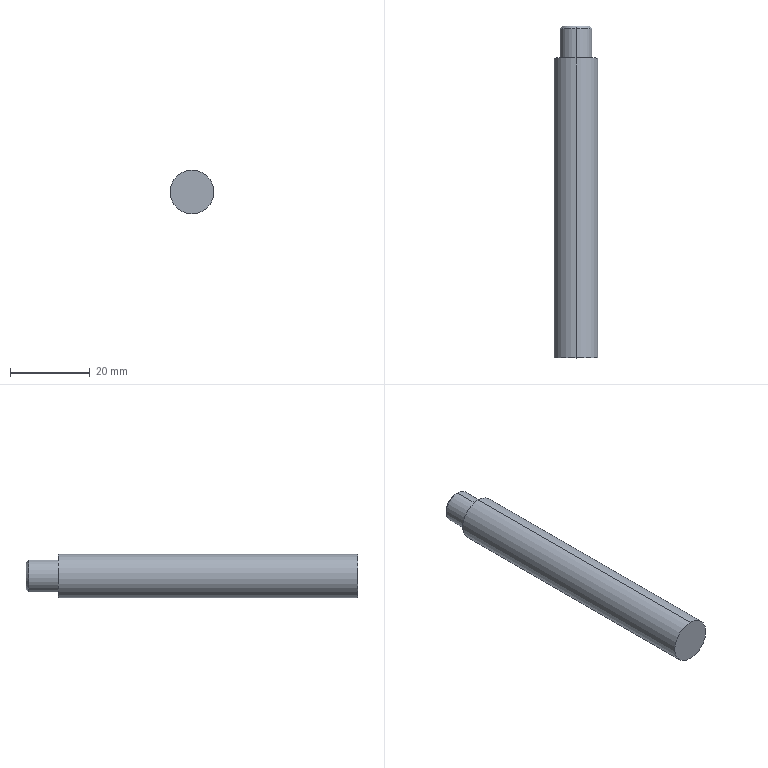Part | SolidWorks | features Extrusion 1, ICE 1, StudWizard 1 | 1 solid | 9 faces | box 11 x 83 x 11 mm | volume 7524 mm3 | cylinder 4 | plane 3 | cone 2 | commonest cylinder face diameters 8 x2 11 x2
STEP:
#1=CARTESIAN_POINT('',(0.,83.,-3.309));
#2=VERTEX_POINT('',#1);
#3=CARTESIAN_POINT('',(0.,83.,3.309));
#4=VERTEX_POINT('',#3);
#5=CARTESIAN_POINT('',(0.,83.,0.));
#6=DIRECTION('',(0.,-1.,0.));
#7=DIRECTION('',(0.,0.,-1.));
#8=AXIS2_PLACEMENT_3D('',#5,#6,#7);
#9=CIRCLE('',#8,3.309);
#10=EDGE_CURVE('',#2,#4,#9,.T.);
#11=ORIENTED_EDGE('',*,*,#10,.T.);
#12=CARTESIAN_POINT('',(0.,82.31,4.));
#13=VERTEX_POINT('',#12);
#14=CARTESIAN_POINT('',(0.,83.,3.309));
#15=DIRECTION('',(0.,-0.7071,0.7071));
#16=VECTOR('',#15,1000.);
#17=LINE('',#14,#16);
#18=EDGE_CURVE('',#4,#13,#17,.T.);
#19=ORIENTED_EDGE('',*,*,#18,.T.);
#20=CARTESIAN_POINT('',(0.,82.31,-4.));
#21=VERTEX_POINT('',#20);
#22=CARTESIAN_POINT('',(0.,82.31,0.));
#23=DIRECTION('',(0.,-1.,0.));
#24=DIRECTION('',(0.,0.,-1.));
#25=AXIS2_PLACEMENT_3D('',#22,#23,#24);
#26=CIRCLE('',#25,4.);
#27=EDGE_CURVE('',#21,#13,#26,.T.);
#28=ORIENTED_EDGE('',*,*,#27,.F.);
#29=CARTESIAN_POINT('',(0.,83.,-3.309));
#30=DIRECTION('',(0.,-0.7071,-0.7071));
#31=VECTOR('',#30,1000.);
#32=LINE('',#29,#31);
#33=EDGE_CURVE('',#2,#21,#32,.T.);
#34=ORIENTED_EDGE('',*,*,#33,.F.);
#35=EDGE_LOOP('',(#11,#19,#28,#34));
#36=FACE_OUTER_BOUND('',#35,.T.);
#37=CARTESIAN_POINT('',(0.,83.,0.));
#38=DIRECTION('',(0.,-1.,0.));
#39=DIRECTION('',(0.,0.,-1.));
#40=AXIS2_PLACEMENT_3D('',#37,#38,#39);
#41=CONICAL_SURFACE('',#40,3.309,0.7854);
#42=ADVANCED_FACE('',(#36),#41,.T.);
#43=ORIENTED_EDGE('',*,*,#27,.T.);
#44=CARTESIAN_POINT('',(0.,75.,4.));
#45=VERTEX_POINT('',#44);
#46=CARTESIAN_POINT('',(0.,83.,4.));
#47=DIRECTION('',(0.,-1.,0.));
#48=VECTOR('',#47,1000.);
#49=LINE('',#46,#48);
#50=EDGE_CURVE('',#13,#45,#49,.T.);
#51=ORIENTED_EDGE('',*,*,#50,.T.);
#52=CARTESIAN_POINT('',(0.,75.,-4.));
#53=VERTEX_POINT('',#52);
#54=CARTESIAN_POINT('',(0.,75.,0.));
#55=DIRECTION('',(0.,1.,0.));
#56=DIRECTION('',(0.,0.,1.));
#57=AXIS2_PLACEMENT_3D('',#54,#55,#56);
#58=CIRCLE('',#57,4.);
#59=EDGE_CURVE('',#45,#53,#58,.T.);
#60=ORIENTED_EDGE('',*,*,#59,.T.);
#61=CARTESIAN_POINT('',(0.,83.,-4.));
#62=DIRECTION('',(0.,-1.,0.));
#63=VECTOR('',#62,1000.);
#64=LINE('',#61,#63);
#65=EDGE_CURVE('',#21,#53,#64,.T.);
#66=ORIENTED_EDGE('',*,*,#65,.F.);
#67=EDGE_LOOP('',(#43,#51,#60,#66));
#68=FACE_OUTER_BOUND('',#67,.T.);
#69=CARTESIAN_POINT('',(0.,83.,0.));
#70=DIRECTION('',(0.,-1.,0.));
#71=DIRECTION('',(0.,0.,-1.));
#72=AXIS2_PLACEMENT_3D('',#69,#70,#71);
#73=CYLINDRICAL_SURFACE('',#72,4.);
#74=ADVANCED_FACE('',(#68),#73,.T.);
#75=CARTESIAN_POINT('',(0.,75.,5.5));
#76=VERTEX_POINT('',#75);
#77=CARTESIAN_POINT('',(0.,75.,-5.5));
#78=VERTEX_POINT('',#77);
#79=CARTESIAN_POINT('',(0.,75.,0.));
#80=DIRECTION('',(0.,1.,0.));
#81=DIRECTION('',(0.,0.,1.));
#82=AXIS2_PLACEMENT_3D('',#79,#80,#81);
#83=CIRCLE('',#82,5.5);
#84=EDGE_CURVE('',#76,#78,#83,.T.);
#85=ORIENTED_EDGE('',*,*,#84,.F.);
#86=CARTESIAN_POINT('',(0.,0.,5.5));
#87=VERTEX_POINT('',#86);
#88=CARTESIAN_POINT('',(0.,75.,5.5));
#89=DIRECTION('',(0.,-1.,0.));
#90=VECTOR('',#89,1000.);
#91=LINE('',#88,#90);
#92=EDGE_CURVE('',#76,#87,#91,.T.);
#93=ORIENTED_EDGE('',*,*,#92,.T.);
#94=CARTESIAN_POINT('',(0.,0.,-5.5));
#95=VERTEX_POINT('',#94);
#96=CARTESIAN_POINT('',(0.,0.,0.));
#97=DIRECTION('',(0.,1.,0.));
#98=DIRECTION('',(0.,0.,1.));
#99=AXIS2_PLACEMENT_3D('',#96,#97,#98);
#100=CIRCLE('',#99,5.5);
#101=EDGE_CURVE('',#87,#95,#100,.T.);
#102=ORIENTED_EDGE('',*,*,#101,.T.);
#103=CARTESIAN_POINT('',(0.,75.,-5.5));
#104=DIRECTION('',(0.,-1.,0.));
#105=VECTOR('',#104,1000.);
#106=LINE('',#103,#105);
#107=EDGE_CURVE('',#78,#95,#106,.T.);
#108=ORIENTED_EDGE('',*,*,#107,.F.);
#109=EDGE_LOOP('',(#85,#93,#102,#108));
#110=FACE_OUTER_BOUND('',#109,.T.);
#111=CARTESIAN_POINT('',(0.,75.,0.));
#112=DIRECTION('',(0.,-1.,0.));
#113=DIRECTION('',(0.,0.,-1.));
#114=AXIS2_PLACEMENT_3D('',#111,#112,#113);
#115=CYLINDRICAL_SURFACE('',#114,5.5);
#116=ADVANCED_FACE('',(#110),#115,.T.);
#117=ORIENTED_EDGE('',*,*,#92,.F.);
#118=CARTESIAN_POINT('',(0.,75.,0.));
#119=DIRECTION('',(0.,1.,0.));
#120=DIRECTION('',(0.,0.,1.));
#121=AXIS2_PLACEMENT_3D('',#118,#119,#120);
#122=CIRCLE('',#121,5.5);
#123=EDGE_CURVE('',#78,#76,#122,.T.);
#124=ORIENTED_EDGE('',*,*,#123,.F.);
#125=ORIENTED_EDGE('',*,*,#107,.T.);
#126=CARTESIAN_POINT('',(0.,0.,0.));
#127=DIRECTION('',(0.,1.,0.));
#128=DIRECTION('',(0.,0.,1.));
#129=AXIS2_PLACEMENT_3D('',#126,#127,#128);
#130=CIRCLE('',#129,5.5);
#131=EDGE_CURVE('',#95,#87,#130,.T.);
#132=ORIENTED_EDGE('',*,*,#131,.T.);
#133=EDGE_LOOP('',(#117,#124,#125,#132));
#134=FACE_OUTER_BOUND('',#133,.T.);
#135=CARTESIAN_POINT('',(0.,75.,0.));
#136=DIRECTION('',(0.,-1.,0.));
#137=DIRECTION('',(0.,0.,-1.));
#138=AXIS2_PLACEMENT_3D('',#135,#136,#137);
#139=CYLINDRICAL_SURFACE('',#138,5.5);
#140=ADVANCED_FACE('',(#134),#139,.T.);
#141=CARTESIAN_POINT('',(0.,75.,0.));
#142=DIRECTION('',(0.,1.,0.));
#143=DIRECTION('',(0.,0.,1.));
#144=AXIS2_PLACEMENT_3D('',#141,#142,#143);
#145=CIRCLE('',#144,4.);
#146=EDGE_CURVE('',#53,#45,#145,.T.);
#147=ORIENTED_EDGE('',*,*,#146,.F.);
#148=ORIENTED_EDGE('',*,*,#59,.F.);
#149=EDGE_LOOP('',(#147,#148));
#150=FACE_BOUND('',#149,.T.);
#151=ORIENTED_EDGE('',*,*,#123,.T.);
#152=ORIENTED_EDGE('',*,*,#84,.T.);
#153=EDGE_LOOP('',(#151,#152));
#154=FACE_OUTER_BOUND('',#153,.T.);
#155=CARTESIAN_POINT('',(0.,75.,0.));
#156=DIRECTION('',(0.,1.,0.));
#157=DIRECTION('',(0.,0.,1.));
#158=AXIS2_PLACEMENT_3D('',#155,#156,#157);
#159=PLANE('',#158);
#160=ADVANCED_FACE('',(#150,#154),#159,.T.);
#161=ORIENTED_EDGE('',*,*,#131,.F.);
#162=ORIENTED_EDGE('',*,*,#101,.F.);
#163=EDGE_LOOP('',(#161,#162));
#164=FACE_OUTER_BOUND('',#163,.T.);
#165=CARTESIAN_POINT('',(0.,0.,0.));
#166=DIRECTION('',(0.,1.,0.));
#167=DIRECTION('',(0.,0.,1.));
#168=AXIS2_PLACEMENT_3D('',#165,#166,#167);
#169=PLANE('',#168);
#170=ADVANCED_FACE('',(#164),#169,.F.);
#171=ORIENTED_EDGE('',*,*,#50,.F.);
#172=CARTESIAN_POINT('',(0.,82.31,0.));
#173=DIRECTION('',(0.,-1.,0.));
#174=DIRECTION('',(0.,0.,-1.));
#175=AXIS2_PLACEMENT_3D('',#172,#173,#174);
#176=CIRCLE('',#175,4.);
#177=EDGE_CURVE('',#13,#21,#176,.T.);
#178=ORIENTED_EDGE('',*,*,#177,.T.);
#179=ORIENTED_EDGE('',*,*,#65,.T.);
#180=ORIENTED_EDGE('',*,*,#146,.T.);
#181=EDGE_LOOP('',(#171,#178,#179,#180));
#182=FACE_OUTER_BOUND('',#181,.T.);
#183=CARTESIAN_POINT('',(0.,83.,0.));
#184=DIRECTION('',(0.,-1.,0.));
#185=DIRECTION('',(0.,0.,-1.));
#186=AXIS2_PLACEMENT_3D('',#183,#184,#185);
#187=CYLINDRICAL_SURFACE('',#186,4.);
#188=ADVANCED_FACE('',(#182),#187,.T.);
#189=ORIENTED_EDGE('',*,*,#18,.F.);
#190=CARTESIAN_POINT('',(0.,83.,0.));
#191=DIRECTION('',(0.,-1.,0.));
#192=DIRECTION('',(0.,0.,-1.));
#193=AXIS2_PLACEMENT_3D('',#190,#191,#192);
#194=CIRCLE('',#193,3.309);
#195=EDGE_CURVE('',#4,#2,#194,.T.);
#196=ORIENTED_EDGE('',*,*,#195,.T.);
#197=ORIENTED_EDGE('',*,*,#33,.T.);
#198=ORIENTED_EDGE('',*,*,#177,.F.);
#199=EDGE_LOOP('',(#189,#196,#197,#198));
#200=FACE_OUTER_BOUND('',#199,.T.);
#201=CARTESIAN_POINT('',(0.,83.,0.));
#202=DIRECTION('',(0.,-1.,0.));
#203=DIRECTION('',(0.,0.,-1.));
#204=AXIS2_PLACEMENT_3D('',#201,#202,#203);
#205=CONICAL_SURFACE('',#204,3.309,0.7854);
#206=ADVANCED_FACE('',(#200),#205,.T.);
#207=ORIENTED_EDGE('',*,*,#10,.F.);
#208=ORIENTED_EDGE('',*,*,#195,.F.);
#209=EDGE_LOOP('',(#207,#208));
#210=FACE_OUTER_BOUND('',#209,.T.);
#211=CARTESIAN_POINT('',(0.,83.,0.));
#212=DIRECTION('',(0.,1.,0.));
#213=DIRECTION('',(0.,0.,1.));
#214=AXIS2_PLACEMENT_3D('',#211,#212,#213);
#215=PLANE('',#214);
#216=ADVANCED_FACE('',(#210),#215,.T.);
#217=CLOSED_SHELL('',(#42,#74,#116,#140,#160,#170,#188,#206,#216));
#218=MANIFOLD_SOLID_BREP('',#217);
#219=CARTESIAN_POINT('',(0.,0.,0.));
#220=DIRECTION('',(0.,0.,1.));
#221=DIRECTION('',(1.,0.,0.));
#222=AXIS2_PLACEMENT_3D('',#219,#220,#221);
#223=(LENGTH_UNIT()NAMED_UNIT(*)SI_UNIT(.MILLI.,.METRE.));
#224=UNCERTAINTY_MEASURE_WITH_UNIT(LENGTH_MEASURE(0.00001),#223,'','');
#225=(NAMED_UNIT(*)PLANE_ANGLE_UNIT()SI_UNIT($,.RADIAN.));
#226=(NAMED_UNIT(*)SI_UNIT($,.STERADIAN.)SOLID_ANGLE_UNIT());
#227=(GEOMETRIC_REPRESENTATION_CONTEXT(3)GLOBAL_UNCERTAINTY_ASSIGNED_CONTEXT((#224))GLOBAL_UNIT_ASSIGNED_CONTEXT((#223,#225,#226))REPRESENTATION_CONTEXT('',''));
#228=ADVANCED_BREP_SHAPE_REPRESENTATION('',(#218,#222),#227);